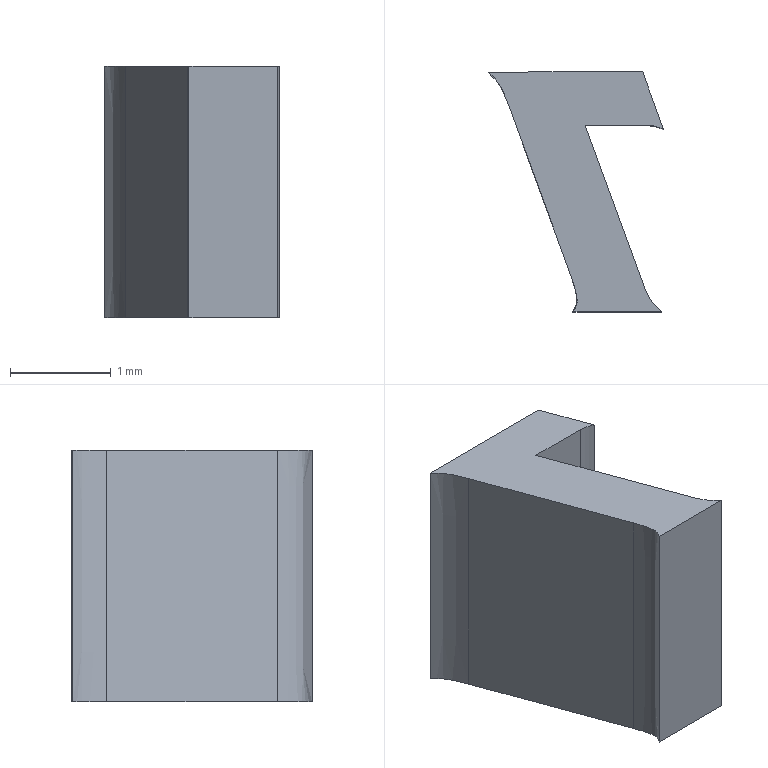Part | STEP file | lll_id1090_x_t | 1 solid | 12 faces | box 1.742 x 2.385 x 2.5 mm | volume 5.148 mm3 | plane 7 | cylinder 3 | other 2 | commonest cylinder face diameters 0.565 x1 0.83 x1 203.505 x1
STEP:
#1=CARTESIAN_POINT('',(386.03,-126.066,2.35));
#2=VERTEX_POINT('',#1);
#3=CARTESIAN_POINT('',(385.878,-126.025,2.35));
#4=VERTEX_POINT('',#3);
#5=CARTESIAN_POINT('',(385.879,-126.307,2.35));
#6=DIRECTION('',(0.,0.,1.));
#7=DIRECTION('',(-1.,0.,0.));
#8=AXIS2_PLACEMENT_3D('',#5,#6,#7);
#9=CIRCLE('',#8,0.2824);
#10=EDGE_CURVE('',#2,#4,#9,.T.);
#11=ORIENTED_EDGE('',*,*,#10,.T.);
#12=CARTESIAN_POINT('',(385.878,-126.025,-0.15));
#13=VERTEX_POINT('',#12);
#14=CARTESIAN_POINT('',(385.878,-126.025,-0.15));
#15=DIRECTION('',(0.,0.,1.));
#16=VECTOR('',#15,1.);
#17=LINE('',#14,#16);
#18=EDGE_CURVE('',#13,#4,#17,.T.);
#19=ORIENTED_EDGE('',*,*,#18,.F.);
#20=CARTESIAN_POINT('',(386.03,-126.066,-0.15));
#21=VERTEX_POINT('',#20);
#22=CARTESIAN_POINT('',(385.879,-126.307,-0.15));
#23=DIRECTION('',(0.,0.,1.));
#24=DIRECTION('',(-1.,0.,0.));
#25=AXIS2_PLACEMENT_3D('',#22,#23,#24);
#26=CIRCLE('',#25,0.2824);
#27=EDGE_CURVE('',#21,#13,#26,.T.);
#28=ORIENTED_EDGE('',*,*,#27,.F.);
#29=CARTESIAN_POINT('',(386.034,-126.071,-0.15));
#30=DIRECTION('',(0.,0.,1.));
#31=VECTOR('',#30,1.);
#32=LINE('',#29,#31);
#33=EDGE_CURVE('',#21,#2,#32,.T.);
#34=ORIENTED_EDGE('',*,*,#33,.T.);
#35=EDGE_LOOP('',(#11,#19,#28,#34));
#36=FACE_OUTER_BOUND('',#35,.T.);
#37=CARTESIAN_POINT('',(385.879,-126.307,-0.15));
#38=DIRECTION('',(0.,0.,1.));
#39=DIRECTION('',(1.,0.,0.));
#40=AXIS2_PLACEMENT_3D('',#37,#38,#39);
#41=CYLINDRICAL_SURFACE('',#40,0.2824);
#42=ADVANCED_FACE('',(#36),#41,.F.);
#43=CARTESIAN_POINT('',(385.251,-126.023,2.35));
#44=VERTEX_POINT('',#43);
#45=CARTESIAN_POINT('',(385.878,-126.025,2.35));
#46=DIRECTION('',(-1.,0.003567,0.));
#47=VECTOR('',#46,1.);
#48=LINE('',#45,#47);
#49=EDGE_CURVE('',#4,#44,#48,.T.);
#50=ORIENTED_EDGE('',*,*,#49,.T.);
#51=CARTESIAN_POINT('',(385.251,-126.023,-0.15));
#52=VERTEX_POINT('',#51);
#53=CARTESIAN_POINT('',(385.251,-126.023,-0.15));
#54=DIRECTION('',(0.,0.,1.));
#55=VECTOR('',#54,1.);
#56=LINE('',#53,#55);
#57=EDGE_CURVE('',#52,#44,#56,.T.);
#58=ORIENTED_EDGE('',*,*,#57,.F.);
#59=CARTESIAN_POINT('',(385.878,-126.025,-0.15));
#60=DIRECTION('',(-1.,0.003567,0.));
#61=VECTOR('',#60,1.);
#62=LINE('',#59,#61);
#63=EDGE_CURVE('',#13,#52,#62,.T.);
#64=ORIENTED_EDGE('',*,*,#63,.F.);
#65=ORIENTED_EDGE('',*,*,#18,.T.);
#66=EDGE_LOOP('',(#50,#58,#64,#65));
#67=FACE_OUTER_BOUND('',#66,.T.);
#68=CARTESIAN_POINT('',(385.878,-126.025,-0.15));
#69=DIRECTION('',(0.003567,1.,0.));
#70=DIRECTION('',(1.,-0.003567,0.));
#71=AXIS2_PLACEMENT_3D('',#68,#69,#70);
#72=PLANE('',#71);
#73=ADVANCED_FACE('',(#67),#72,.F.);
#74=CARTESIAN_POINT('',(385.853,-127.665,2.35));
#75=VERTEX_POINT('',#74);
#76=CARTESIAN_POINT('',(385.251,-126.023,2.35));
#77=DIRECTION('',(0.344,-0.939,0.));
#78=VECTOR('',#77,1.);
#79=LINE('',#76,#78);
#80=EDGE_CURVE('',#44,#75,#79,.T.);
#81=ORIENTED_EDGE('',*,*,#80,.T.);
#82=CARTESIAN_POINT('',(385.853,-127.665,-0.15));
#83=VERTEX_POINT('',#82);
#84=CARTESIAN_POINT('',(385.853,-127.665,-0.15));
#85=DIRECTION('',(0.,0.,1.));
#86=VECTOR('',#85,1.);
#87=LINE('',#84,#86);
#88=EDGE_CURVE('',#83,#75,#87,.T.);
#89=ORIENTED_EDGE('',*,*,#88,.F.);
#90=CARTESIAN_POINT('',(385.251,-126.023,-0.15));
#91=DIRECTION('',(0.344,-0.939,0.));
#92=VECTOR('',#91,1.);
#93=LINE('',#90,#92);
#94=EDGE_CURVE('',#52,#83,#93,.T.);
#95=ORIENTED_EDGE('',*,*,#94,.F.);
#96=ORIENTED_EDGE('',*,*,#57,.T.);
#97=EDGE_LOOP('',(#81,#89,#95,#96));
#98=FACE_OUTER_BOUND('',#97,.T.);
#99=CARTESIAN_POINT('',(385.251,-126.023,-0.15));
#100=DIRECTION('',(-0.939,-0.344,0.));
#101=DIRECTION('',(-0.344,0.939,0.));
#102=AXIS2_PLACEMENT_3D('',#99,#100,#101);
#103=PLANE('',#102);
#104=ADVANCED_FACE('',(#98),#103,.F.);
#105=CARTESIAN_POINT('',(386.014,-127.874,2.35));
#106=VERTEX_POINT('',#105);
#107=CARTESIAN_POINT('',(386.244,-127.525,2.35));
#108=DIRECTION('',(0.,0.,1.));
#109=DIRECTION('',(-1.,0.,0.));
#110=AXIS2_PLACEMENT_3D('',#107,#108,#109);
#111=CIRCLE('',#110,0.4149);
#112=EDGE_CURVE('',#75,#106,#111,.T.);
#113=ORIENTED_EDGE('',*,*,#112,.T.);
#114=CARTESIAN_POINT('',(386.014,-127.874,-0.15));
#115=VERTEX_POINT('',#114);
#116=CARTESIAN_POINT('',(386.022,-127.876,-0.15));
#117=DIRECTION('',(0.,0.,1.));
#118=VECTOR('',#117,1.);
#119=LINE('',#116,#118);
#120=EDGE_CURVE('',#115,#106,#119,.T.);
#121=ORIENTED_EDGE('',*,*,#120,.F.);
#122=CARTESIAN_POINT('',(386.244,-127.525,-0.15));
#123=DIRECTION('',(0.,0.,1.));
#124=DIRECTION('',(-1.,0.,0.));
#125=AXIS2_PLACEMENT_3D('',#122,#123,#124);
#126=CIRCLE('',#125,0.4149);
#127=EDGE_CURVE('',#83,#115,#126,.T.);
#128=ORIENTED_EDGE('',*,*,#127,.F.);
#129=ORIENTED_EDGE('',*,*,#88,.T.);
#130=EDGE_LOOP('',(#113,#121,#128,#129));
#131=FACE_OUTER_BOUND('',#130,.T.);
#132=CARTESIAN_POINT('',(386.244,-127.525,-0.15));
#133=DIRECTION('',(0.,0.,1.));
#134=DIRECTION('',(1.,0.,0.));
#135=AXIS2_PLACEMENT_3D('',#132,#133,#134);
#136=CYLINDRICAL_SURFACE('',#135,0.4149);
#137=ADVANCED_FACE('',(#131),#136,.F.);
#138=CARTESIAN_POINT('',(385.131,-127.876,2.35));
#139=VERTEX_POINT('',#138);
#140=CARTESIAN_POINT('',(386.013,-127.876,2.35));
#141=DIRECTION('',(-1.,0.,0.));
#142=VECTOR('',#141,1.);
#143=LINE('',#140,#142);
#144=EDGE_CURVE('',#106,#139,#143,.T.);
#145=ORIENTED_EDGE('',*,*,#144,.T.);
#146=CARTESIAN_POINT('',(385.131,-127.876,-0.15));
#147=VERTEX_POINT('',#146);
#148=CARTESIAN_POINT('',(385.131,-127.876,-0.15));
#149=DIRECTION('',(0.,0.,1.));
#150=VECTOR('',#149,1.);
#151=LINE('',#148,#150);
#152=EDGE_CURVE('',#147,#139,#151,.T.);
#153=ORIENTED_EDGE('',*,*,#152,.F.);
#154=CARTESIAN_POINT('',(386.013,-127.876,-0.15));
#155=DIRECTION('',(-1.,0.,0.));
#156=VECTOR('',#155,1.);
#157=LINE('',#154,#156);
#158=EDGE_CURVE('',#115,#147,#157,.T.);
#159=ORIENTED_EDGE('',*,*,#158,.F.);
#160=ORIENTED_EDGE('',*,*,#120,.T.);
#161=EDGE_LOOP('',(#145,#153,#159,#160));
#162=FACE_OUTER_BOUND('',#161,.T.);
#163=CARTESIAN_POINT('',(386.013,-127.876,-0.15));
#164=DIRECTION('',(0.,1.,0.));
#165=DIRECTION('',(0.,0.,1.));
#166=AXIS2_PLACEMENT_3D('',#163,#164,#165);
#167=PLANE('',#166);
#168=ADVANCED_FACE('',(#162),#167,.F.);
#169=CARTESIAN_POINT('',(385.115,-127.533,2.35));
#170=VERTEX_POINT('',#169);
#171=CARTESIAN_POINT('',(385.131,-127.876,2.35));
#172=CARTESIAN_POINT('',(385.153,-127.85,2.35));
#173=CARTESIAN_POINT('',(385.167,-127.819,2.35));
#174=CARTESIAN_POINT('',(385.172,-127.77,2.35));
#175=CARTESIAN_POINT('',(385.172,-127.754,2.35));
#176=CARTESIAN_POINT('',(385.17,-127.732,2.35));
#177=CARTESIAN_POINT('',(385.169,-127.725,2.35));
#178=CARTESIAN_POINT('',(385.166,-127.706,2.35));
#179=CARTESIAN_POINT('',(385.164,-127.695,2.35));
#180=CARTESIAN_POINT('',(385.159,-127.673,2.35));
#181=CARTESIAN_POINT('',(385.157,-127.662,2.35));
#182=CARTESIAN_POINT('',(385.15,-127.64,2.35));
#183=CARTESIAN_POINT('',(385.147,-127.629,2.35));
#184=CARTESIAN_POINT('',(385.135,-127.59,2.35));
#185=CARTESIAN_POINT('',(385.126,-127.561,2.35));
#186=CARTESIAN_POINT('',(385.115,-127.533,2.35));
#187=(BOUNDED_CURVE()B_SPLINE_CURVE(3,(#171,#172,#173,#174,#175,#176,#177,#178,#179,#180,#181,#182,#183,#184,#185,#186),.UNSPECIFIED.,.F.,.F.)B_SPLINE_CURVE_WITH_KNOTS((4,2,2,2,2,2,2,4),(0.,0.2854,0.41,0.472,0.5649,0.6582,0.7514,1.),.UNSPECIFIED.)CURVE()GEOMETRIC_REPRESENTATION_ITEM()RATIONAL_B_SPLINE_CURVE((0.5118,0.4961,0.4961,0.5102,0.5102,0.5115,0.5115,0.5115,0.5115,0.5116,0.5116,0.5117,0.5117,0.5116,0.5116,0.5118))REPRESENTATION_ITEM(''));
#188=EDGE_CURVE('',#139,#170,#187,.T.);
#189=ORIENTED_EDGE('',*,*,#188,.T.);
#190=CARTESIAN_POINT('',(385.115,-127.533,-0.15));
#191=VERTEX_POINT('',#190);
#192=CARTESIAN_POINT('',(385.115,-127.533,-0.15));
#193=DIRECTION('',(0.,0.,1.));
#194=VECTOR('',#193,1.);
#195=LINE('',#192,#194);
#196=EDGE_CURVE('',#191,#170,#195,.T.);
#197=ORIENTED_EDGE('',*,*,#196,.F.);
#198=CARTESIAN_POINT('',(385.131,-127.876,-0.15));
#199=CARTESIAN_POINT('',(385.153,-127.85,-0.15));
#200=CARTESIAN_POINT('',(385.167,-127.819,-0.15));
#201=CARTESIAN_POINT('',(385.172,-127.77,-0.15));
#202=CARTESIAN_POINT('',(385.172,-127.754,-0.15));
#203=CARTESIAN_POINT('',(385.17,-127.732,-0.15));
#204=CARTESIAN_POINT('',(385.169,-127.725,-0.15));
#205=CARTESIAN_POINT('',(385.166,-127.706,-0.15));
#206=CARTESIAN_POINT('',(385.164,-127.695,-0.15));
#207=CARTESIAN_POINT('',(385.159,-127.673,-0.15));
#208=CARTESIAN_POINT('',(385.157,-127.662,-0.15));
#209=CARTESIAN_POINT('',(385.15,-127.64,-0.15));
#210=CARTESIAN_POINT('',(385.147,-127.629,-0.15));
#211=CARTESIAN_POINT('',(385.135,-127.59,-0.15));
#212=CARTESIAN_POINT('',(385.126,-127.561,-0.15));
#213=CARTESIAN_POINT('',(385.115,-127.533,-0.15));
#214=(BOUNDED_CURVE()B_SPLINE_CURVE(3,(#198,#199,#200,#201,#202,#203,#204,#205,#206,#207,#208,#209,#210,#211,#212,#213),.UNSPECIFIED.,.F.,.F.)B_SPLINE_CURVE_WITH_KNOTS((4,2,2,2,2,2,2,4),(0.,0.2854,0.41,0.472,0.5649,0.6582,0.7514,1.),.UNSPECIFIED.)CURVE()GEOMETRIC_REPRESENTATION_ITEM()RATIONAL_B_SPLINE_CURVE((0.5118,0.4961,0.4961,0.5102,0.5102,0.5115,0.5115,0.5115,0.5115,0.5116,0.5116,0.5117,0.5117,0.5116,0.5116,0.5118))REPRESENTATION_ITEM(''));
#215=EDGE_CURVE('',#147,#191,#214,.T.);
#216=ORIENTED_EDGE('',*,*,#215,.F.);
#217=ORIENTED_EDGE('',*,*,#152,.T.);
#218=EDGE_LOOP('',(#189,#197,#216,#217));
#219=FACE_OUTER_BOUND('',#218,.T.);
#220=CARTESIAN_POINT('',(385.131,-127.876,-0.15));
#221=CARTESIAN_POINT('',(385.153,-127.85,-0.15));
#222=CARTESIAN_POINT('',(385.167,-127.819,-0.15));
#223=CARTESIAN_POINT('',(385.172,-127.77,-0.15));
#224=CARTESIAN_POINT('',(385.172,-127.754,-0.15));
#225=CARTESIAN_POINT('',(385.17,-127.732,-0.15));
#226=CARTESIAN_POINT('',(385.169,-127.725,-0.15));
#227=CARTESIAN_POINT('',(385.166,-127.706,-0.15));
#228=CARTESIAN_POINT('',(385.164,-127.695,-0.15));
#229=CARTESIAN_POINT('',(385.159,-127.673,-0.15));
#230=CARTESIAN_POINT('',(385.157,-127.662,-0.15));
#231=CARTESIAN_POINT('',(385.15,-127.64,-0.15));
#232=CARTESIAN_POINT('',(385.147,-127.629,-0.15));
#233=CARTESIAN_POINT('',(385.135,-127.59,-0.15));
#234=CARTESIAN_POINT('',(385.126,-127.561,-0.15));
#235=CARTESIAN_POINT('',(385.115,-127.533,-0.15));
#236=(BOUNDED_CURVE()B_SPLINE_CURVE(3,(#220,#221,#222,#223,#224,#225,#226,#227,#228,#229,#230,#231,#232,#233,#234,#235),.UNSPECIFIED.,.F.,.F.)B_SPLINE_CURVE_WITH_KNOTS((4,2,2,2,2,2,2,4),(0.,0.2854,0.41,0.472,0.5649,0.6582,0.7514,1.),.UNSPECIFIED.)CURVE()GEOMETRIC_REPRESENTATION_ITEM()RATIONAL_B_SPLINE_CURVE((0.5118,0.4961,0.4961,0.5102,0.5102,0.5115,0.5115,0.5115,0.5115,0.5116,0.5116,0.5117,0.5117,0.5116,0.5116,0.5118))REPRESENTATION_ITEM(''));
#237=DIRECTION('',(0.,0.,1.));
#238=VECTOR('',#237,1.);
#239=SURFACE_OF_LINEAR_EXTRUSION('',#236,#238);
#240=ADVANCED_FACE('',(#219),#239,.F.);
#241=CARTESIAN_POINT('',(384.497,-125.836,2.35));
#242=VERTEX_POINT('',#241);
#243=CARTESIAN_POINT('',(385.115,-127.533,2.35));
#244=DIRECTION('',(-0.3421,0.9397,0.));
#245=VECTOR('',#244,1.);
#246=LINE('',#243,#245);
#247=EDGE_CURVE('',#170,#242,#246,.T.);
#248=ORIENTED_EDGE('',*,*,#247,.T.);
#249=CARTESIAN_POINT('',(384.497,-125.836,-0.15));
#250=VERTEX_POINT('',#249);
#251=CARTESIAN_POINT('',(384.497,-125.836,-0.15));
#252=DIRECTION('',(0.,0.,1.));
#253=VECTOR('',#252,1.);
#254=LINE('',#251,#253);
#255=EDGE_CURVE('',#250,#242,#254,.T.);
#256=ORIENTED_EDGE('',*,*,#255,.F.);
#257=CARTESIAN_POINT('',(385.115,-127.533,-0.15));
#258=DIRECTION('',(-0.3421,0.9397,0.));
#259=VECTOR('',#258,1.);
#260=LINE('',#257,#259);
#261=EDGE_CURVE('',#191,#250,#260,.T.);
#262=ORIENTED_EDGE('',*,*,#261,.F.);
#263=ORIENTED_EDGE('',*,*,#196,.T.);
#264=EDGE_LOOP('',(#248,#256,#262,#263));
#265=FACE_OUTER_BOUND('',#264,.T.);
#266=CARTESIAN_POINT('',(385.115,-127.533,-0.15));
#267=DIRECTION('',(0.9397,0.3421,0.));
#268=DIRECTION('',(0.3421,-0.9397,0.));
#269=AXIS2_PLACEMENT_3D('',#266,#267,#268);
#270=PLANE('',#269);
#271=ADVANCED_FACE('',(#265),#270,.F.);
#272=CARTESIAN_POINT('',(384.292,-125.498,2.35));
#273=VERTEX_POINT('',#272);
#274=CARTESIAN_POINT('',(384.497,-125.836,2.35));
#275=CARTESIAN_POINT('',(384.492,-125.82,2.35));
#276=CARTESIAN_POINT('',(384.486,-125.804,2.35));
#277=CARTESIAN_POINT('',(384.47,-125.761,2.35));
#278=CARTESIAN_POINT('',(384.458,-125.734,2.35));
#279=CARTESIAN_POINT('',(384.438,-125.689,2.35));
#280=CARTESIAN_POINT('',(384.429,-125.67,2.35));
#281=CARTESIAN_POINT('',(384.407,-125.629,2.35));
#282=CARTESIAN_POINT('',(384.393,-125.608,2.35));
#283=CARTESIAN_POINT('',(384.354,-125.554,2.35));
#284=CARTESIAN_POINT('',(384.325,-125.524,2.35));
#285=CARTESIAN_POINT('',(384.292,-125.498,2.35));
#286=(BOUNDED_CURVE()B_SPLINE_CURVE(3,(#274,#275,#276,#277,#278,#279,#280,#281,#282,#283,#284,#285),.UNSPECIFIED.,.F.,.F.)B_SPLINE_CURVE_WITH_KNOTS((4,2,2,2,2,4),(0.,0.1253,0.3445,0.5009,0.6886,1.),.UNSPECIFIED.)CURVE()GEOMETRIC_REPRESENTATION_ITEM()RATIONAL_B_SPLINE_CURVE((0.5,0.5,0.5,0.4998,0.4998,0.4998,0.4998,0.4993,0.4993,0.4971,0.4971,0.5))REPRESENTATION_ITEM(''));
#287=EDGE_CURVE('',#242,#273,#286,.T.);
#288=ORIENTED_EDGE('',*,*,#287,.T.);
#289=CARTESIAN_POINT('',(384.292,-125.498,-0.15));
#290=VERTEX_POINT('',#289);
#291=CARTESIAN_POINT('',(384.292,-125.498,-0.15));
#292=DIRECTION('',(0.,0.,1.));
#293=VECTOR('',#292,1.);
#294=LINE('',#291,#293);
#295=EDGE_CURVE('',#290,#273,#294,.T.);
#296=ORIENTED_EDGE('',*,*,#295,.F.);
#297=CARTESIAN_POINT('',(384.497,-125.836,-0.15));
#298=CARTESIAN_POINT('',(384.492,-125.82,-0.15));
#299=CARTESIAN_POINT('',(384.486,-125.804,-0.15));
#300=CARTESIAN_POINT('',(384.47,-125.761,-0.15));
#301=CARTESIAN_POINT('',(384.458,-125.734,-0.15));
#302=CARTESIAN_POINT('',(384.438,-125.689,-0.15));
#303=CARTESIAN_POINT('',(384.429,-125.67,-0.15));
#304=CARTESIAN_POINT('',(384.407,-125.629,-0.15));
#305=CARTESIAN_POINT('',(384.393,-125.608,-0.15));
#306=CARTESIAN_POINT('',(384.354,-125.554,-0.15));
#307=CARTESIAN_POINT('',(384.325,-125.524,-0.15));
#308=CARTESIAN_POINT('',(384.292,-125.498,-0.15));
#309=(BOUNDED_CURVE()B_SPLINE_CURVE(3,(#297,#298,#299,#300,#301,#302,#303,#304,#305,#306,#307,#308),.UNSPECIFIED.,.F.,.F.)B_SPLINE_CURVE_WITH_KNOTS((4,2,2,2,2,4),(0.,0.1253,0.3445,0.5009,0.6886,1.),.UNSPECIFIED.)CURVE()GEOMETRIC_REPRESENTATION_ITEM()RATIONAL_B_SPLINE_CURVE((0.5,0.5,0.5,0.4998,0.4998,0.4998,0.4998,0.4993,0.4993,0.4971,0.4971,0.5))REPRESENTATION_ITEM(''));
#310=EDGE_CURVE('',#250,#290,#309,.T.);
#311=ORIENTED_EDGE('',*,*,#310,.F.);
#312=ORIENTED_EDGE('',*,*,#255,.T.);
#313=EDGE_LOOP('',(#288,#296,#311,#312));
#314=FACE_OUTER_BOUND('',#313,.T.);
#315=CARTESIAN_POINT('',(384.497,-125.836,-0.15));
#316=CARTESIAN_POINT('',(384.492,-125.82,-0.15));
#317=CARTESIAN_POINT('',(384.486,-125.804,-0.15));
#318=CARTESIAN_POINT('',(384.47,-125.761,-0.15));
#319=CARTESIAN_POINT('',(384.458,-125.734,-0.15));
#320=CARTESIAN_POINT('',(384.438,-125.689,-0.15));
#321=CARTESIAN_POINT('',(384.429,-125.67,-0.15));
#322=CARTESIAN_POINT('',(384.407,-125.629,-0.15));
#323=CARTESIAN_POINT('',(384.393,-125.608,-0.15));
#324=CARTESIAN_POINT('',(384.354,-125.554,-0.15));
#325=CARTESIAN_POINT('',(384.325,-125.524,-0.15));
#326=CARTESIAN_POINT('',(384.292,-125.498,-0.15));
#327=(BOUNDED_CURVE()B_SPLINE_CURVE(3,(#315,#316,#317,#318,#319,#320,#321,#322,#323,#324,#325,#326),.UNSPECIFIED.,.F.,.F.)B_SPLINE_CURVE_WITH_KNOTS((4,2,2,2,2,4),(0.,0.1253,0.3445,0.5009,0.6886,1.),.UNSPECIFIED.)CURVE()GEOMETRIC_REPRESENTATION_ITEM()RATIONAL_B_SPLINE_CURVE((0.5,0.5,0.5,0.4998,0.4998,0.4998,0.4998,0.4993,0.4993,0.4971,0.4971,0.5))REPRESENTATION_ITEM(''));
#328=DIRECTION('',(0.,0.,1.));
#329=VECTOR('',#328,1.);
#330=SURFACE_OF_LINEAR_EXTRUSION('',#327,#329);
#331=ADVANCED_FACE('',(#314),#330,.F.);
#332=CARTESIAN_POINT('',(385.823,-125.492,2.35));
#333=VERTEX_POINT('',#332);
#334=CARTESIAN_POINT('',(385.419,-227.244,2.35));
#335=DIRECTION('',(0.,0.,-1.));
#336=DIRECTION('',(-1.,0.,0.));
#337=AXIS2_PLACEMENT_3D('',#334,#335,#336);
#338=CIRCLE('',#337,101.752);
#339=EDGE_CURVE('',#273,#333,#338,.T.);
#340=ORIENTED_EDGE('',*,*,#339,.T.);
#341=CARTESIAN_POINT('',(385.823,-125.492,-0.15));
#342=VERTEX_POINT('',#341);
#343=CARTESIAN_POINT('',(385.823,-125.492,-0.15));
#344=DIRECTION('',(0.,0.,1.));
#345=VECTOR('',#344,1.);
#346=LINE('',#343,#345);
#347=EDGE_CURVE('',#342,#333,#346,.T.);
#348=ORIENTED_EDGE('',*,*,#347,.F.);
#349=CARTESIAN_POINT('',(385.419,-227.244,-0.15));
#350=DIRECTION('',(0.,0.,-1.));
#351=DIRECTION('',(-1.,0.,0.));
#352=AXIS2_PLACEMENT_3D('',#349,#350,#351);
#353=CIRCLE('',#352,101.752);
#354=EDGE_CURVE('',#290,#342,#353,.T.);
#355=ORIENTED_EDGE('',*,*,#354,.F.);
#356=ORIENTED_EDGE('',*,*,#295,.T.);
#357=EDGE_LOOP('',(#340,#348,#355,#356));
#358=FACE_OUTER_BOUND('',#357,.T.);
#359=CARTESIAN_POINT('',(385.419,-227.244,-0.15));
#360=DIRECTION('',(0.,0.,1.));
#361=DIRECTION('',(1.,0.,0.));
#362=AXIS2_PLACEMENT_3D('',#359,#360,#361);
#363=CYLINDRICAL_SURFACE('',#362,101.752);
#364=ADVANCED_FACE('',(#358),#363,.T.);
#365=CARTESIAN_POINT('',(385.823,-125.492,2.35));
#366=DIRECTION('',(0.3426,-0.9395,0.));
#367=VECTOR('',#366,1.);
#368=LINE('',#365,#367);
#369=EDGE_CURVE('',#333,#2,#368,.T.);
#370=ORIENTED_EDGE('',*,*,#369,.T.);
#371=ORIENTED_EDGE('',*,*,#33,.F.);
#372=CARTESIAN_POINT('',(385.823,-125.492,-0.15));
#373=DIRECTION('',(0.3426,-0.9395,0.));
#374=VECTOR('',#373,1.);
#375=LINE('',#372,#374);
#376=EDGE_CURVE('',#342,#21,#375,.T.);
#377=ORIENTED_EDGE('',*,*,#376,.F.);
#378=ORIENTED_EDGE('',*,*,#347,.T.);
#379=EDGE_LOOP('',(#370,#371,#377,#378));
#380=FACE_OUTER_BOUND('',#379,.T.);
#381=CARTESIAN_POINT('',(385.823,-125.492,-0.15));
#382=DIRECTION('',(-0.9395,-0.3426,0.));
#383=DIRECTION('',(-0.3426,0.9395,0.));
#384=AXIS2_PLACEMENT_3D('',#381,#382,#383);
#385=PLANE('',#384);
#386=ADVANCED_FACE('',(#380),#385,.F.);
#387=ORIENTED_EDGE('',*,*,#27,.T.);
#388=ORIENTED_EDGE('',*,*,#63,.T.);
#389=ORIENTED_EDGE('',*,*,#94,.T.);
#390=ORIENTED_EDGE('',*,*,#127,.T.);
#391=ORIENTED_EDGE('',*,*,#158,.T.);
#392=ORIENTED_EDGE('',*,*,#215,.T.);
#393=ORIENTED_EDGE('',*,*,#261,.T.);
#394=ORIENTED_EDGE('',*,*,#310,.T.);
#395=ORIENTED_EDGE('',*,*,#354,.T.);
#396=ORIENTED_EDGE('',*,*,#376,.T.);
#397=EDGE_LOOP('',(#387,#388,#389,#390,#391,#392,#393,#394,#395,#396));
#398=FACE_OUTER_BOUND('',#397,.T.);
#399=CARTESIAN_POINT('',(385.879,-126.307,-0.15));
#400=DIRECTION('',(0.,0.,1.));
#401=DIRECTION('',(1.,0.,0.));
#402=AXIS2_PLACEMENT_3D('',#399,#400,#401);
#403=PLANE('',#402);
#404=ADVANCED_FACE('',(#398),#403,.F.);
#405=ORIENTED_EDGE('',*,*,#10,.F.);
#406=ORIENTED_EDGE('',*,*,#369,.F.);
#407=ORIENTED_EDGE('',*,*,#339,.F.);
#408=ORIENTED_EDGE('',*,*,#287,.F.);
#409=ORIENTED_EDGE('',*,*,#247,.F.);
#410=ORIENTED_EDGE('',*,*,#188,.F.);
#411=ORIENTED_EDGE('',*,*,#144,.F.);
#412=ORIENTED_EDGE('',*,*,#112,.F.);
#413=ORIENTED_EDGE('',*,*,#80,.F.);
#414=ORIENTED_EDGE('',*,*,#49,.F.);
#415=EDGE_LOOP('',(#405,#406,#407,#408,#409,#410,#411,#412,#413,#414));
#416=FACE_OUTER_BOUND('',#415,.T.);
#417=CARTESIAN_POINT('',(385.879,-126.307,2.35));
#418=DIRECTION('',(0.,0.,1.));
#419=DIRECTION('',(1.,0.,0.));
#420=AXIS2_PLACEMENT_3D('',#417,#418,#419);
#421=PLANE('',#420);
#422=ADVANCED_FACE('',(#416),#421,.T.);
#423=CLOSED_SHELL('',(#42,#73,#104,#137,#168,#240,#271,#331,#364,#386,#404,#422));
#424=MANIFOLD_SOLID_BREP('',#423);
#425=(LENGTH_UNIT()NAMED_UNIT(*)SI_UNIT(.MILLI.,.METRE.));
#426=UNCERTAINTY_MEASURE_WITH_UNIT(LENGTH_MEASURE(0.0184),#425,'','');
#427=(NAMED_UNIT(*)PLANE_ANGLE_UNIT()SI_UNIT($,.RADIAN.));
#428=PLANE_ANGLE_MEASURE_WITH_UNIT(PLANE_ANGLE_MEASURE(0.01745),#427);
#429=DIMENSIONAL_EXPONENTS(0.,0.,0.,0.,0.,0.,0.);
#430=(CONVERSION_BASED_UNIT('DEGREE',#428)NAMED_UNIT(#429)PLANE_ANGLE_UNIT());
#431=(NAMED_UNIT(*)SI_UNIT($,.STERADIAN.)SOLID_ANGLE_UNIT());
#432=(GEOMETRIC_REPRESENTATION_CONTEXT(3)GLOBAL_UNCERTAINTY_ASSIGNED_CONTEXT((#426))GLOBAL_UNIT_ASSIGNED_CONTEXT((#425,#430,#431))REPRESENTATION_CONTEXT('',''));
#433=ADVANCED_BREP_SHAPE_REPRESENTATION('',(#424),#432);